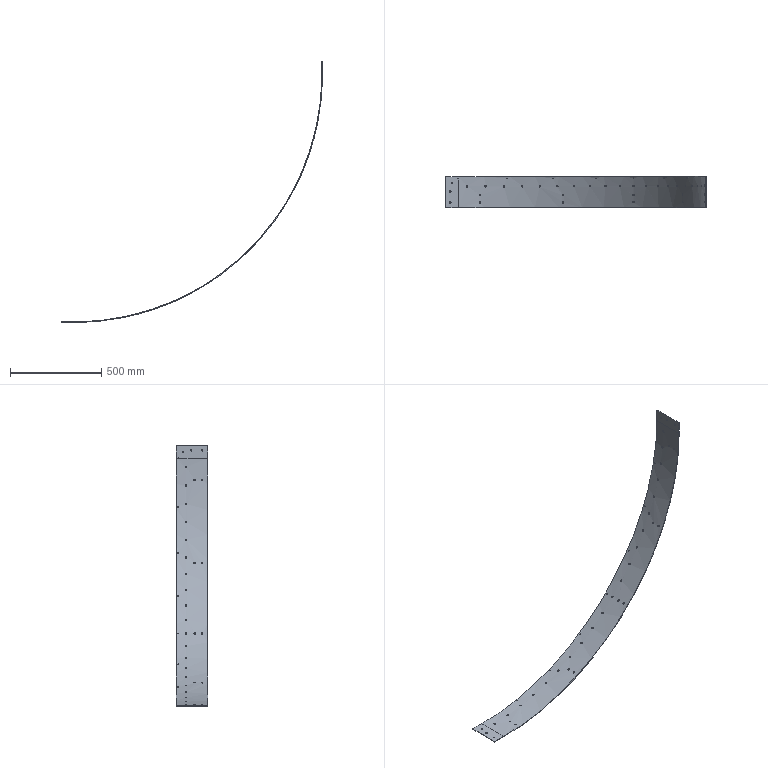Part | STEP file | curverollersoutside | 1 solid | 134 faces | box 1429 x 170 x 1429 mm | volume 959320 mm3 | spline 59 | cone 43 | cylinder 24 | plane 8 | commonest cylinder face diameters 9 x17 4.917 x5 2712 x1 2717 x1